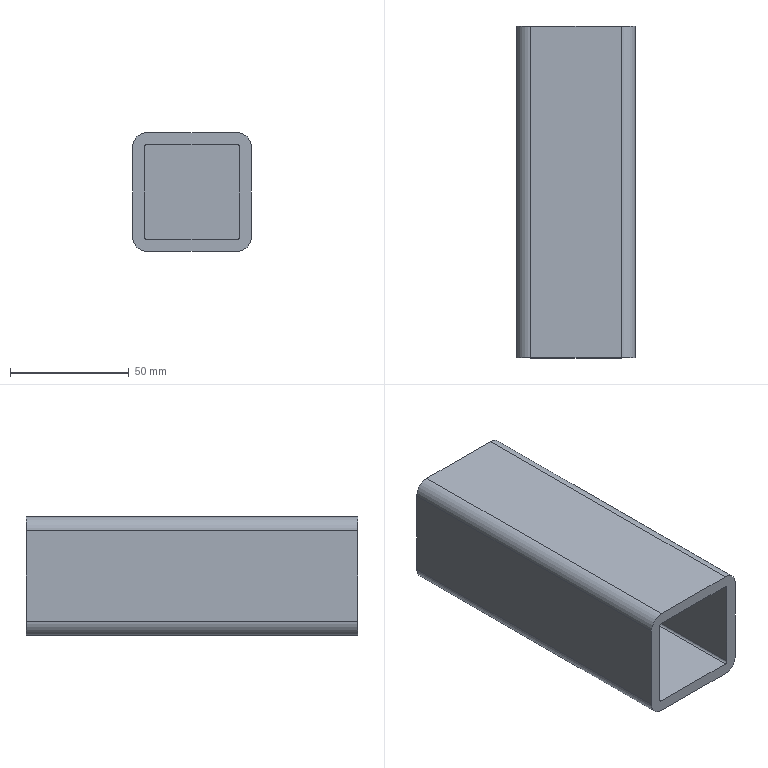Part | SolidWorks | features Extrusion 1, ICE 1 | 1 solid | 19 faces | box 50 x 140 x 50 mm | volume 129790 mm3 | plane 11 | cylinder 8 | commonest cylinder face diameters 2 x4 12 x4
STEP:
#1=CARTESIAN_POINT('',(-20.,135.,6.278));
#2=VERTEX_POINT('',#1);
#3=CARTESIAN_POINT('',(-20.,0.,6.278));
#4=VERTEX_POINT('',#3);
#5=CARTESIAN_POINT('',(-20.,140.,6.278));
#6=DIRECTION('',(0.,-1.,0.));
#7=VECTOR('',#6,1000.);
#8=LINE('',#5,#7);
#9=EDGE_CURVE('',#2,#4,#8,.T.);
#10=ORIENTED_EDGE('',*,*,#9,.F.);
#11=CARTESIAN_POINT('',(-19.,135.,7.278));
#12=VERTEX_POINT('',#11);
#13=CARTESIAN_POINT('',(-19.,135.,6.278));
#14=DIRECTION('',(0.,1.,0.));
#15=DIRECTION('',(0.,0.,1.));
#16=AXIS2_PLACEMENT_3D('',#13,#14,#15);
#17=CIRCLE('',#16,1.);
#18=EDGE_CURVE('',#2,#12,#17,.T.);
#19=ORIENTED_EDGE('',*,*,#18,.T.);
#20=CARTESIAN_POINT('',(-19.,0.,7.278));
#21=VERTEX_POINT('',#20);
#22=CARTESIAN_POINT('',(-19.,140.,7.278));
#23=DIRECTION('',(0.,-1.,0.));
#24=VECTOR('',#23,1000.);
#25=LINE('',#22,#24);
#26=EDGE_CURVE('',#12,#21,#25,.T.);
#27=ORIENTED_EDGE('',*,*,#26,.T.);
#28=CARTESIAN_POINT('',(-19.,0.,6.278));
#29=DIRECTION('',(0.,1.,0.));
#30=DIRECTION('',(0.,0.,-1.));
#31=AXIS2_PLACEMENT_3D('',#28,#29,#30);
#32=CIRCLE('',#31,1.);
#33=EDGE_CURVE('',#4,#21,#32,.T.);
#34=ORIENTED_EDGE('',*,*,#33,.F.);
#35=EDGE_LOOP('',(#10,#19,#27,#34));
#36=FACE_OUTER_BOUND('',#35,.T.);
#37=CARTESIAN_POINT('',(-19.,140.,6.278));
#38=DIRECTION('',(0.,-1.,0.));
#39=DIRECTION('',(0.,0.,-1.));
#40=AXIS2_PLACEMENT_3D('',#37,#38,#39);
#41=CYLINDRICAL_SURFACE('',#40,1.);
#42=ADVANCED_FACE('',(#36),#41,.F.);
#43=ORIENTED_EDGE('',*,*,#26,.F.);
#44=CARTESIAN_POINT('',(19.,135.,7.278));
#45=VERTEX_POINT('',#44);
#46=CARTESIAN_POINT('',(-19.,135.,7.278));
#47=DIRECTION('',(1.,0.,0.));
#48=VECTOR('',#47,1000.);
#49=LINE('',#46,#48);
#50=EDGE_CURVE('',#12,#45,#49,.T.);
#51=ORIENTED_EDGE('',*,*,#50,.T.);
#52=CARTESIAN_POINT('',(19.,0.,7.278));
#53=VERTEX_POINT('',#52);
#54=CARTESIAN_POINT('',(19.,140.,7.278));
#55=DIRECTION('',(0.,-1.,0.));
#56=VECTOR('',#55,1000.);
#57=LINE('',#54,#56);
#58=EDGE_CURVE('',#45,#53,#57,.T.);
#59=ORIENTED_EDGE('',*,*,#58,.T.);
#60=CARTESIAN_POINT('',(-19.,0.,7.278));
#61=DIRECTION('',(1.,0.,0.));
#62=VECTOR('',#61,1000.);
#63=LINE('',#60,#62);
#64=EDGE_CURVE('',#21,#53,#63,.T.);
#65=ORIENTED_EDGE('',*,*,#64,.F.);
#66=EDGE_LOOP('',(#43,#51,#59,#65));
#67=FACE_OUTER_BOUND('',#66,.T.);
#68=CARTESIAN_POINT('',(-19.,140.,7.278));
#69=DIRECTION('',(0.,0.,-1.));
#70=DIRECTION('',(-1.,0.,0.));
#71=AXIS2_PLACEMENT_3D('',#68,#69,#70);
#72=PLANE('',#71);
#73=ADVANCED_FACE('',(#67),#72,.T.);
#74=ORIENTED_EDGE('',*,*,#58,.F.);
#75=CARTESIAN_POINT('',(20.,135.,6.278));
#76=VERTEX_POINT('',#75);
#77=CARTESIAN_POINT('',(19.,135.,6.278));
#78=DIRECTION('',(0.,1.,0.));
#79=DIRECTION('',(0.,0.,1.));
#80=AXIS2_PLACEMENT_3D('',#77,#78,#79);
#81=CIRCLE('',#80,1.);
#82=EDGE_CURVE('',#45,#76,#81,.T.);
#83=ORIENTED_EDGE('',*,*,#82,.T.);
#84=CARTESIAN_POINT('',(20.,0.,6.278));
#85=VERTEX_POINT('',#84);
#86=CARTESIAN_POINT('',(20.,140.,6.278));
#87=DIRECTION('',(0.,-1.,0.));
#88=VECTOR('',#87,1000.);
#89=LINE('',#86,#88);
#90=EDGE_CURVE('',#76,#85,#89,.T.);
#91=ORIENTED_EDGE('',*,*,#90,.T.);
#92=CARTESIAN_POINT('',(19.,0.,6.278));
#93=DIRECTION('',(0.,1.,0.));
#94=DIRECTION('',(0.,0.,1.));
#95=AXIS2_PLACEMENT_3D('',#92,#93,#94);
#96=CIRCLE('',#95,1.);
#97=EDGE_CURVE('',#53,#85,#96,.T.);
#98=ORIENTED_EDGE('',*,*,#97,.F.);
#99=EDGE_LOOP('',(#74,#83,#91,#98));
#100=FACE_OUTER_BOUND('',#99,.T.);
#101=CARTESIAN_POINT('',(19.,140.,6.278));
#102=DIRECTION('',(0.,-1.,0.));
#103=DIRECTION('',(0.,0.,-1.));
#104=AXIS2_PLACEMENT_3D('',#101,#102,#103);
#105=CYLINDRICAL_SURFACE('',#104,1.);
#106=ADVANCED_FACE('',(#100),#105,.F.);
#107=ORIENTED_EDGE('',*,*,#90,.F.);
#108=CARTESIAN_POINT('',(20.,135.,-31.722));
#109=VERTEX_POINT('',#108);
#110=CARTESIAN_POINT('',(20.,135.,6.278));
#111=DIRECTION('',(0.,0.,-1.));
#112=VECTOR('',#111,1000.);
#113=LINE('',#110,#112);
#114=EDGE_CURVE('',#76,#109,#113,.T.);
#115=ORIENTED_EDGE('',*,*,#114,.T.);
#116=CARTESIAN_POINT('',(20.,0.,-31.722));
#117=VERTEX_POINT('',#116);
#118=CARTESIAN_POINT('',(20.,140.,-31.722));
#119=DIRECTION('',(0.,-1.,0.));
#120=VECTOR('',#119,1000.);
#121=LINE('',#118,#120);
#122=EDGE_CURVE('',#109,#117,#121,.T.);
#123=ORIENTED_EDGE('',*,*,#122,.T.);
#124=CARTESIAN_POINT('',(20.,0.,6.278));
#125=DIRECTION('',(0.,0.,-1.));
#126=VECTOR('',#125,1000.);
#127=LINE('',#124,#126);
#128=EDGE_CURVE('',#85,#117,#127,.T.);
#129=ORIENTED_EDGE('',*,*,#128,.F.);
#130=EDGE_LOOP('',(#107,#115,#123,#129));
#131=FACE_OUTER_BOUND('',#130,.T.);
#132=CARTESIAN_POINT('',(20.,140.,6.278));
#133=DIRECTION('',(-1.,0.,0.));
#134=DIRECTION('',(0.,0.,1.));
#135=AXIS2_PLACEMENT_3D('',#132,#133,#134);
#136=PLANE('',#135);
#137=ADVANCED_FACE('',(#131),#136,.T.);
#138=ORIENTED_EDGE('',*,*,#122,.F.);
#139=CARTESIAN_POINT('',(19.,135.,-32.722));
#140=VERTEX_POINT('',#139);
#141=CARTESIAN_POINT('',(19.,135.,-31.722));
#142=DIRECTION('',(0.,1.,0.));
#143=DIRECTION('',(0.,0.,1.));
#144=AXIS2_PLACEMENT_3D('',#141,#142,#143);
#145=CIRCLE('',#144,1.);
#146=EDGE_CURVE('',#109,#140,#145,.T.);
#147=ORIENTED_EDGE('',*,*,#146,.T.);
#148=CARTESIAN_POINT('',(19.,0.,-32.722));
#149=VERTEX_POINT('',#148);
#150=CARTESIAN_POINT('',(19.,140.,-32.722));
#151=DIRECTION('',(0.,-1.,0.));
#152=VECTOR('',#151,1000.);
#153=LINE('',#150,#152);
#154=EDGE_CURVE('',#140,#149,#153,.T.);
#155=ORIENTED_EDGE('',*,*,#154,.T.);
#156=CARTESIAN_POINT('',(19.,0.,-31.722));
#157=DIRECTION('',(0.,1.,0.));
#158=DIRECTION('',(0.,0.,-1.));
#159=AXIS2_PLACEMENT_3D('',#156,#157,#158);
#160=CIRCLE('',#159,1.);
#161=EDGE_CURVE('',#117,#149,#160,.T.);
#162=ORIENTED_EDGE('',*,*,#161,.F.);
#163=EDGE_LOOP('',(#138,#147,#155,#162));
#164=FACE_OUTER_BOUND('',#163,.T.);
#165=CARTESIAN_POINT('',(19.,140.,-31.722));
#166=DIRECTION('',(0.,-1.,0.));
#167=DIRECTION('',(0.,0.,-1.));
#168=AXIS2_PLACEMENT_3D('',#165,#166,#167);
#169=CYLINDRICAL_SURFACE('',#168,1.);
#170=ADVANCED_FACE('',(#164),#169,.F.);
#171=ORIENTED_EDGE('',*,*,#154,.F.);
#172=CARTESIAN_POINT('',(-19.,135.,-32.722));
#173=VERTEX_POINT('',#172);
#174=CARTESIAN_POINT('',(-19.,135.,-32.722));
#175=DIRECTION('',(-1.,0.,0.));
#176=VECTOR('',#175,1000.);
#177=LINE('',#174,#176);
#178=EDGE_CURVE('',#140,#173,#177,.T.);
#179=ORIENTED_EDGE('',*,*,#178,.T.);
#180=CARTESIAN_POINT('',(-19.,0.,-32.722));
#181=VERTEX_POINT('',#180);
#182=CARTESIAN_POINT('',(-19.,140.,-32.722));
#183=DIRECTION('',(0.,-1.,0.));
#184=VECTOR('',#183,1000.);
#185=LINE('',#182,#184);
#186=EDGE_CURVE('',#173,#181,#185,.T.);
#187=ORIENTED_EDGE('',*,*,#186,.T.);
#188=CARTESIAN_POINT('',(-19.,0.,-32.722));
#189=DIRECTION('',(-1.,0.,0.));
#190=VECTOR('',#189,1000.);
#191=LINE('',#188,#190);
#192=EDGE_CURVE('',#149,#181,#191,.T.);
#193=ORIENTED_EDGE('',*,*,#192,.F.);
#194=EDGE_LOOP('',(#171,#179,#187,#193));
#195=FACE_OUTER_BOUND('',#194,.T.);
#196=CARTESIAN_POINT('',(-19.,140.,-32.722));
#197=DIRECTION('',(0.,0.,1.));
#198=DIRECTION('',(1.,0.,0.));
#199=AXIS2_PLACEMENT_3D('',#196,#197,#198);
#200=PLANE('',#199);
#201=ADVANCED_FACE('',(#195),#200,.T.);
#202=ORIENTED_EDGE('',*,*,#186,.F.);
#203=CARTESIAN_POINT('',(-20.,135.,-31.722));
#204=VERTEX_POINT('',#203);
#205=CARTESIAN_POINT('',(-19.,135.,-31.722));
#206=DIRECTION('',(0.,1.,0.));
#207=DIRECTION('',(0.,0.,1.));
#208=AXIS2_PLACEMENT_3D('',#205,#206,#207);
#209=CIRCLE('',#208,1.);
#210=EDGE_CURVE('',#173,#204,#209,.T.);
#211=ORIENTED_EDGE('',*,*,#210,.T.);
#212=CARTESIAN_POINT('',(-20.,0.,-31.722));
#213=VERTEX_POINT('',#212);
#214=CARTESIAN_POINT('',(-20.,140.,-31.722));
#215=DIRECTION('',(0.,-1.,0.));
#216=VECTOR('',#215,1000.);
#217=LINE('',#214,#216);
#218=EDGE_CURVE('',#204,#213,#217,.T.);
#219=ORIENTED_EDGE('',*,*,#218,.T.);
#220=CARTESIAN_POINT('',(-19.,0.,-31.722));
#221=DIRECTION('',(0.,1.,0.));
#222=DIRECTION('',(0.,0.,-1.));
#223=AXIS2_PLACEMENT_3D('',#220,#221,#222);
#224=CIRCLE('',#223,1.);
#225=EDGE_CURVE('',#181,#213,#224,.T.);
#226=ORIENTED_EDGE('',*,*,#225,.F.);
#227=EDGE_LOOP('',(#202,#211,#219,#226));
#228=FACE_OUTER_BOUND('',#227,.T.);
#229=CARTESIAN_POINT('',(-19.,140.,-31.722));
#230=DIRECTION('',(0.,-1.,0.));
#231=DIRECTION('',(0.,0.,-1.));
#232=AXIS2_PLACEMENT_3D('',#229,#230,#231);
#233=CYLINDRICAL_SURFACE('',#232,1.);
#234=ADVANCED_FACE('',(#228),#233,.F.);
#235=ORIENTED_EDGE('',*,*,#218,.F.);
#236=CARTESIAN_POINT('',(-20.,135.,6.278));
#237=DIRECTION('',(0.,0.,1.));
#238=VECTOR('',#237,1000.);
#239=LINE('',#236,#238);
#240=EDGE_CURVE('',#204,#2,#239,.T.);
#241=ORIENTED_EDGE('',*,*,#240,.T.);
#242=ORIENTED_EDGE('',*,*,#9,.T.);
#243=CARTESIAN_POINT('',(-20.,0.,6.278));
#244=DIRECTION('',(0.,0.,1.));
#245=VECTOR('',#244,1000.);
#246=LINE('',#243,#245);
#247=EDGE_CURVE('',#213,#4,#246,.T.);
#248=ORIENTED_EDGE('',*,*,#247,.F.);
#249=EDGE_LOOP('',(#235,#241,#242,#248));
#250=FACE_OUTER_BOUND('',#249,.T.);
#251=CARTESIAN_POINT('',(-20.,140.,6.278));
#252=DIRECTION('',(1.,0.,0.));
#253=DIRECTION('',(0.,0.,-1.));
#254=AXIS2_PLACEMENT_3D('',#251,#252,#253);
#255=PLANE('',#254);
#256=ADVANCED_FACE('',(#250),#255,.T.);
#257=CARTESIAN_POINT('',(-25.,140.,6.278));
#258=VERTEX_POINT('',#257);
#259=CARTESIAN_POINT('',(-19.,140.,12.278));
#260=VERTEX_POINT('',#259);
#261=CARTESIAN_POINT('',(-19.,140.,6.278));
#262=DIRECTION('',(0.,1.,0.));
#263=DIRECTION('',(0.,0.,-1.));
#264=AXIS2_PLACEMENT_3D('',#261,#262,#263);
#265=CIRCLE('',#264,6.);
#266=EDGE_CURVE('',#258,#260,#265,.T.);
#267=ORIENTED_EDGE('',*,*,#266,.T.);
#268=CARTESIAN_POINT('',(19.,140.,12.278));
#269=VERTEX_POINT('',#268);
#270=CARTESIAN_POINT('',(-19.,140.,12.278));
#271=DIRECTION('',(1.,0.,0.));
#272=VECTOR('',#271,1000.);
#273=LINE('',#270,#272);
#274=EDGE_CURVE('',#260,#269,#273,.T.);
#275=ORIENTED_EDGE('',*,*,#274,.T.);
#276=CARTESIAN_POINT('',(25.,140.,6.278));
#277=VERTEX_POINT('',#276);
#278=CARTESIAN_POINT('',(19.,140.,6.278));
#279=DIRECTION('',(0.,1.,0.));
#280=DIRECTION('',(0.,0.,1.));
#281=AXIS2_PLACEMENT_3D('',#278,#279,#280);
#282=CIRCLE('',#281,6.);
#283=EDGE_CURVE('',#269,#277,#282,.T.);
#284=ORIENTED_EDGE('',*,*,#283,.T.);
#285=CARTESIAN_POINT('',(25.,140.,-31.722));
#286=VERTEX_POINT('',#285);
#287=CARTESIAN_POINT('',(25.,140.,6.278));
#288=DIRECTION('',(0.,0.,-1.));
#289=VECTOR('',#288,1000.);
#290=LINE('',#287,#289);
#291=EDGE_CURVE('',#277,#286,#290,.T.);
#292=ORIENTED_EDGE('',*,*,#291,.T.);
#293=CARTESIAN_POINT('',(19.,140.,-37.722));
#294=VERTEX_POINT('',#293);
#295=CARTESIAN_POINT('',(19.,140.,-31.722));
#296=DIRECTION('',(0.,1.,0.));
#297=DIRECTION('',(0.,0.,-1.));
#298=AXIS2_PLACEMENT_3D('',#295,#296,#297);
#299=CIRCLE('',#298,6.);
#300=EDGE_CURVE('',#286,#294,#299,.T.);
#301=ORIENTED_EDGE('',*,*,#300,.T.);
#302=CARTESIAN_POINT('',(-19.,140.,-37.722));
#303=VERTEX_POINT('',#302);
#304=CARTESIAN_POINT('',(-19.,140.,-37.722));
#305=DIRECTION('',(-1.,0.,0.));
#306=VECTOR('',#305,1000.);
#307=LINE('',#304,#306);
#308=EDGE_CURVE('',#294,#303,#307,.T.);
#309=ORIENTED_EDGE('',*,*,#308,.T.);
#310=CARTESIAN_POINT('',(-25.,140.,-31.722));
#311=VERTEX_POINT('',#310);
#312=CARTESIAN_POINT('',(-19.,140.,-31.722));
#313=DIRECTION('',(0.,1.,0.));
#314=DIRECTION('',(0.,0.,-1.));
#315=AXIS2_PLACEMENT_3D('',#312,#313,#314);
#316=CIRCLE('',#315,6.);
#317=EDGE_CURVE('',#303,#311,#316,.T.);
#318=ORIENTED_EDGE('',*,*,#317,.T.);
#319=CARTESIAN_POINT('',(-25.,140.,6.278));
#320=DIRECTION('',(0.,0.,1.));
#321=VECTOR('',#320,1000.);
#322=LINE('',#319,#321);
#323=EDGE_CURVE('',#311,#258,#322,.T.);
#324=ORIENTED_EDGE('',*,*,#323,.T.);
#325=EDGE_LOOP('',(#267,#275,#284,#292,#301,#309,#318,#324));
#326=FACE_OUTER_BOUND('',#325,.T.);
#327=CARTESIAN_POINT('',(-19.,140.,6.278));
#328=DIRECTION('',(0.,-1.,0.));
#329=DIRECTION('',(0.,0.,-1.));
#330=AXIS2_PLACEMENT_3D('',#327,#328,#329);
#331=PLANE('',#330);
#332=ADVANCED_FACE('',(#326),#331,.F.);
#333=CARTESIAN_POINT('',(-25.,0.,6.278));
#334=VERTEX_POINT('',#333);
#335=CARTESIAN_POINT('',(-19.,0.,12.278));
#336=VERTEX_POINT('',#335);
#337=CARTESIAN_POINT('',(-19.,0.,6.278));
#338=DIRECTION('',(0.,1.,0.));
#339=DIRECTION('',(0.,0.,-1.));
#340=AXIS2_PLACEMENT_3D('',#337,#338,#339);
#341=CIRCLE('',#340,6.);
#342=EDGE_CURVE('',#334,#336,#341,.T.);
#343=ORIENTED_EDGE('',*,*,#342,.F.);
#344=CARTESIAN_POINT('',(-25.,0.,-31.722));
#345=VERTEX_POINT('',#344);
#346=CARTESIAN_POINT('',(-25.,0.,6.278));
#347=DIRECTION('',(0.,0.,1.));
#348=VECTOR('',#347,1000.);
#349=LINE('',#346,#348);
#350=EDGE_CURVE('',#345,#334,#349,.T.);
#351=ORIENTED_EDGE('',*,*,#350,.F.);
#352=CARTESIAN_POINT('',(-19.,0.,-37.722));
#353=VERTEX_POINT('',#352);
#354=CARTESIAN_POINT('',(-19.,0.,-31.722));
#355=DIRECTION('',(0.,1.,0.));
#356=DIRECTION('',(0.,0.,-1.));
#357=AXIS2_PLACEMENT_3D('',#354,#355,#356);
#358=CIRCLE('',#357,6.);
#359=EDGE_CURVE('',#353,#345,#358,.T.);
#360=ORIENTED_EDGE('',*,*,#359,.F.);
#361=CARTESIAN_POINT('',(19.,0.,-37.722));
#362=VERTEX_POINT('',#361);
#363=CARTESIAN_POINT('',(-19.,0.,-37.722));
#364=DIRECTION('',(-1.,0.,0.));
#365=VECTOR('',#364,1000.);
#366=LINE('',#363,#365);
#367=EDGE_CURVE('',#362,#353,#366,.T.);
#368=ORIENTED_EDGE('',*,*,#367,.F.);
#369=CARTESIAN_POINT('',(25.,0.,-31.722));
#370=VERTEX_POINT('',#369);
#371=CARTESIAN_POINT('',(19.,0.,-31.722));
#372=DIRECTION('',(0.,1.,0.));
#373=DIRECTION('',(0.,0.,-1.));
#374=AXIS2_PLACEMENT_3D('',#371,#372,#373);
#375=CIRCLE('',#374,6.);
#376=EDGE_CURVE('',#370,#362,#375,.T.);
#377=ORIENTED_EDGE('',*,*,#376,.F.);
#378=CARTESIAN_POINT('',(25.,0.,6.278));
#379=VERTEX_POINT('',#378);
#380=CARTESIAN_POINT('',(25.,0.,6.278));
#381=DIRECTION('',(0.,0.,-1.));
#382=VECTOR('',#381,1000.);
#383=LINE('',#380,#382);
#384=EDGE_CURVE('',#379,#370,#383,.T.);
#385=ORIENTED_EDGE('',*,*,#384,.F.);
#386=CARTESIAN_POINT('',(19.,0.,12.278));
#387=VERTEX_POINT('',#386);
#388=CARTESIAN_POINT('',(19.,0.,6.278));
#389=DIRECTION('',(0.,1.,0.));
#390=DIRECTION('',(0.,0.,1.));
#391=AXIS2_PLACEMENT_3D('',#388,#389,#390);
#392=CIRCLE('',#391,6.);
#393=EDGE_CURVE('',#387,#379,#392,.T.);
#394=ORIENTED_EDGE('',*,*,#393,.F.);
#395=CARTESIAN_POINT('',(-19.,0.,12.278));
#396=DIRECTION('',(1.,0.,0.));
#397=VECTOR('',#396,1000.);
#398=LINE('',#395,#397);
#399=EDGE_CURVE('',#336,#387,#398,.T.);
#400=ORIENTED_EDGE('',*,*,#399,.F.);
#401=EDGE_LOOP('',(#343,#351,#360,#368,#377,#385,#394,#400));
#402=FACE_OUTER_BOUND('',#401,.T.);
#403=ORIENTED_EDGE('',*,*,#247,.T.);
#404=ORIENTED_EDGE('',*,*,#33,.T.);
#405=ORIENTED_EDGE('',*,*,#64,.T.);
#406=ORIENTED_EDGE('',*,*,#97,.T.);
#407=ORIENTED_EDGE('',*,*,#128,.T.);
#408=ORIENTED_EDGE('',*,*,#161,.T.);
#409=ORIENTED_EDGE('',*,*,#192,.T.);
#410=ORIENTED_EDGE('',*,*,#225,.T.);
#411=EDGE_LOOP('',(#403,#404,#405,#406,#407,#408,#409,#410));
#412=FACE_BOUND('',#411,.T.);
#413=CARTESIAN_POINT('',(-19.,0.,6.278));
#414=DIRECTION('',(0.,-1.,0.));
#415=DIRECTION('',(0.,0.,-1.));
#416=AXIS2_PLACEMENT_3D('',#413,#414,#415);
#417=PLANE('',#416);
#418=ADVANCED_FACE('',(#402,#412),#417,.T.);
#419=CARTESIAN_POINT('',(-25.,140.,6.278));
#420=DIRECTION('',(0.,-1.,0.));
#421=VECTOR('',#420,1000.);
#422=LINE('',#419,#421);
#423=EDGE_CURVE('',#258,#334,#422,.T.);
#424=ORIENTED_EDGE('',*,*,#423,.T.);
#425=ORIENTED_EDGE('',*,*,#342,.T.);
#426=CARTESIAN_POINT('',(-19.,140.,12.278));
#427=DIRECTION('',(0.,-1.,0.));
#428=VECTOR('',#427,1000.);
#429=LINE('',#426,#428);
#430=EDGE_CURVE('',#260,#336,#429,.T.);
#431=ORIENTED_EDGE('',*,*,#430,.F.);
#432=ORIENTED_EDGE('',*,*,#266,.F.);
#433=EDGE_LOOP('',(#424,#425,#431,#432));
#434=FACE_OUTER_BOUND('',#433,.T.);
#435=CARTESIAN_POINT('',(-19.,140.,6.278));
#436=DIRECTION('',(0.,-1.,0.));
#437=DIRECTION('',(0.,0.,-1.));
#438=AXIS2_PLACEMENT_3D('',#435,#436,#437);
#439=CYLINDRICAL_SURFACE('',#438,6.);
#440=ADVANCED_FACE('',(#434),#439,.T.);
#441=ORIENTED_EDGE('',*,*,#430,.T.);
#442=ORIENTED_EDGE('',*,*,#399,.T.);
#443=CARTESIAN_POINT('',(19.,140.,12.278));
#444=DIRECTION('',(0.,-1.,0.));
#445=VECTOR('',#444,1000.);
#446=LINE('',#443,#445);
#447=EDGE_CURVE('',#269,#387,#446,.T.);
#448=ORIENTED_EDGE('',*,*,#447,.F.);
#449=ORIENTED_EDGE('',*,*,#274,.F.);
#450=EDGE_LOOP('',(#441,#442,#448,#449));
#451=FACE_OUTER_BOUND('',#450,.T.);
#452=CARTESIAN_POINT('',(-19.,140.,12.278));
#453=DIRECTION('',(0.,0.,-1.));
#454=DIRECTION('',(-1.,0.,0.));
#455=AXIS2_PLACEMENT_3D('',#452,#453,#454);
#456=PLANE('',#455);
#457=ADVANCED_FACE('',(#451),#456,.F.);
#458=ORIENTED_EDGE('',*,*,#447,.T.);
#459=ORIENTED_EDGE('',*,*,#393,.T.);
#460=CARTESIAN_POINT('',(25.,140.,6.278));
#461=DIRECTION('',(0.,-1.,0.));
#462=VECTOR('',#461,1000.);
#463=LINE('',#460,#462);
#464=EDGE_CURVE('',#277,#379,#463,.T.);
#465=ORIENTED_EDGE('',*,*,#464,.F.);
#466=ORIENTED_EDGE('',*,*,#283,.F.);
#467=EDGE_LOOP('',(#458,#459,#465,#466));
#468=FACE_OUTER_BOUND('',#467,.T.);
#469=CARTESIAN_POINT('',(19.,140.,6.278));
#470=DIRECTION('',(0.,-1.,0.));
#471=DIRECTION('',(0.,0.,-1.));
#472=AXIS2_PLACEMENT_3D('',#469,#470,#471);
#473=CYLINDRICAL_SURFACE('',#472,6.);
#474=ADVANCED_FACE('',(#468),#473,.T.);
#475=ORIENTED_EDGE('',*,*,#464,.T.);
#476=ORIENTED_EDGE('',*,*,#384,.T.);
#477=CARTESIAN_POINT('',(25.,140.,-31.722));
#478=DIRECTION('',(0.,-1.,0.));
#479=VECTOR('',#478,1000.);
#480=LINE('',#477,#479);
#481=EDGE_CURVE('',#286,#370,#480,.T.);
#482=ORIENTED_EDGE('',*,*,#481,.F.);
#483=ORIENTED_EDGE('',*,*,#291,.F.);
#484=EDGE_LOOP('',(#475,#476,#482,#483));
#485=FACE_OUTER_BOUND('',#484,.T.);
#486=CARTESIAN_POINT('',(25.,140.,6.278));
#487=DIRECTION('',(-1.,0.,0.));
#488=DIRECTION('',(0.,0.,1.));
#489=AXIS2_PLACEMENT_3D('',#486,#487,#488);
#490=PLANE('',#489);
#491=ADVANCED_FACE('',(#485),#490,.F.);
#492=ORIENTED_EDGE('',*,*,#481,.T.);
#493=ORIENTED_EDGE('',*,*,#376,.T.);
#494=CARTESIAN_POINT('',(19.,140.,-37.722));
#495=DIRECTION('',(0.,-1.,0.));
#496=VECTOR('',#495,1000.);
#497=LINE('',#494,#496);
#498=EDGE_CURVE('',#294,#362,#497,.T.);
#499=ORIENTED_EDGE('',*,*,#498,.F.);
#500=ORIENTED_EDGE('',*,*,#300,.F.);
#501=EDGE_LOOP('',(#492,#493,#499,#500));
#502=FACE_OUTER_BOUND('',#501,.T.);
#503=CARTESIAN_POINT('',(19.,140.,-31.722));
#504=DIRECTION('',(0.,-1.,0.));
#505=DIRECTION('',(0.,0.,-1.));
#506=AXIS2_PLACEMENT_3D('',#503,#504,#505);
#507=CYLINDRICAL_SURFACE('',#506,6.);
#508=ADVANCED_FACE('',(#502),#507,.T.);
#509=ORIENTED_EDGE('',*,*,#498,.T.);
#510=ORIENTED_EDGE('',*,*,#367,.T.);
#511=CARTESIAN_POINT('',(-19.,140.,-37.722));
#512=DIRECTION('',(0.,-1.,0.));
#513=VECTOR('',#512,1000.);
#514=LINE('',#511,#513);
#515=EDGE_CURVE('',#303,#353,#514,.T.);
#516=ORIENTED_EDGE('',*,*,#515,.F.);
#517=ORIENTED_EDGE('',*,*,#308,.F.);
#518=EDGE_LOOP('',(#509,#510,#516,#517));
#519=FACE_OUTER_BOUND('',#518,.T.);
#520=CARTESIAN_POINT('',(-19.,140.,-37.722));
#521=DIRECTION('',(0.,0.,1.));
#522=DIRECTION('',(1.,0.,0.));
#523=AXIS2_PLACEMENT_3D('',#520,#521,#522);
#524=PLANE('',#523);
#525=ADVANCED_FACE('',(#519),#524,.F.);
#526=ORIENTED_EDGE('',*,*,#515,.T.);
#527=ORIENTED_EDGE('',*,*,#359,.T.);
#528=CARTESIAN_POINT('',(-25.,140.,-31.722));
#529=DIRECTION('',(0.,-1.,0.));
#530=VECTOR('',#529,1000.);
#531=LINE('',#528,#530);
#532=EDGE_CURVE('',#311,#345,#531,.T.);
#533=ORIENTED_EDGE('',*,*,#532,.F.);
#534=ORIENTED_EDGE('',*,*,#317,.F.);
#535=EDGE_LOOP('',(#526,#527,#533,#534));
#536=FACE_OUTER_BOUND('',#535,.T.);
#537=CARTESIAN_POINT('',(-19.,140.,-31.722));
#538=DIRECTION('',(0.,-1.,0.));
#539=DIRECTION('',(0.,0.,-1.));
#540=AXIS2_PLACEMENT_3D('',#537,#538,#539);
#541=CYLINDRICAL_SURFACE('',#540,6.);
#542=ADVANCED_FACE('',(#536),#541,.T.);
#543=ORIENTED_EDGE('',*,*,#532,.T.);
#544=ORIENTED_EDGE('',*,*,#350,.T.);
#545=ORIENTED_EDGE('',*,*,#423,.F.);
#546=ORIENTED_EDGE('',*,*,#323,.F.);
#547=EDGE_LOOP('',(#543,#544,#545,#546));
#548=FACE_OUTER_BOUND('',#547,.T.);
#549=CARTESIAN_POINT('',(-25.,140.,6.278));
#550=DIRECTION('',(1.,0.,0.));
#551=DIRECTION('',(0.,0.,-1.));
#552=AXIS2_PLACEMENT_3D('',#549,#550,#551);
#553=PLANE('',#552);
#554=ADVANCED_FACE('',(#548),#553,.F.);
#555=ORIENTED_EDGE('',*,*,#18,.F.);
#556=ORIENTED_EDGE('',*,*,#240,.F.);
#557=ORIENTED_EDGE('',*,*,#210,.F.);
#558=ORIENTED_EDGE('',*,*,#178,.F.);
#559=ORIENTED_EDGE('',*,*,#146,.F.);
#560=ORIENTED_EDGE('',*,*,#114,.F.);
#561=ORIENTED_EDGE('',*,*,#82,.F.);
#562=ORIENTED_EDGE('',*,*,#50,.F.);
#563=EDGE_LOOP('',(#555,#556,#557,#558,#559,#560,#561,#562));
#564=FACE_OUTER_BOUND('',#563,.T.);
#565=CARTESIAN_POINT('',(-19.,135.,6.278));
#566=DIRECTION('',(0.,1.,0.));
#567=DIRECTION('',(0.,0.,1.));
#568=AXIS2_PLACEMENT_3D('',#565,#566,#567);
#569=PLANE('',#568);
#570=ADVANCED_FACE('',(#564),#569,.F.);
#571=CLOSED_SHELL('',(#42,#73,#106,#137,#170,#201,#234,#256,#332,#418,#440,#457,#474,#491,#508,#525,#542,#554,#570));
#572=MANIFOLD_SOLID_BREP('',#571);
#573=CARTESIAN_POINT('',(0.,0.,0.));
#574=DIRECTION('',(0.,0.,1.));
#575=DIRECTION('',(1.,0.,0.));
#576=AXIS2_PLACEMENT_3D('',#573,#574,#575);
#577=(LENGTH_UNIT()NAMED_UNIT(*)SI_UNIT(.MILLI.,.METRE.));
#578=UNCERTAINTY_MEASURE_WITH_UNIT(LENGTH_MEASURE(0.00001),#577,'','');
#579=(NAMED_UNIT(*)PLANE_ANGLE_UNIT()SI_UNIT($,.RADIAN.));
#580=(NAMED_UNIT(*)SI_UNIT($,.STERADIAN.)SOLID_ANGLE_UNIT());
#581=(GEOMETRIC_REPRESENTATION_CONTEXT(3)GLOBAL_UNCERTAINTY_ASSIGNED_CONTEXT((#578))GLOBAL_UNIT_ASSIGNED_CONTEXT((#577,#579,#580))REPRESENTATION_CONTEXT('',''));
#582=ADVANCED_BREP_SHAPE_REPRESENTATION('',(#572,#576),#581);